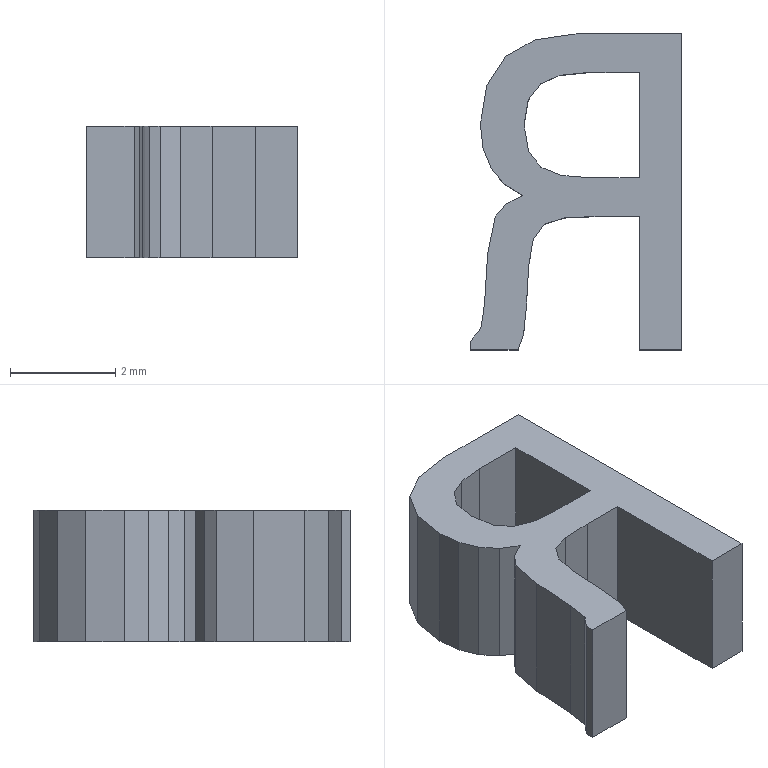Part | STEP file | lll_id1146_x_t | 1 solid | 41 faces | box 4.011 x 6 x 2.5 mm | volume 30.988 mm3 | plane 41
STEP:
#1=CARTESIAN_POINT('',(388.453,102.132,2.35));
#2=VERTEX_POINT('',#1);
#3=CARTESIAN_POINT('',(388.219,101.83,2.35));
#4=VERTEX_POINT('',#3);
#5=CARTESIAN_POINT('',(388.453,102.132,2.35));
#6=DIRECTION('',(-0.6108,-0.7918,0.));
#7=VECTOR('',#6,1.);
#8=LINE('',#5,#7);
#9=EDGE_CURVE('',#2,#4,#8,.T.);
#10=ORIENTED_EDGE('',*,*,#9,.T.);
#11=CARTESIAN_POINT('',(388.219,101.83,-0.15));
#12=VERTEX_POINT('',#11);
#13=CARTESIAN_POINT('',(388.219,101.83,-0.15));
#14=DIRECTION('',(0.,0.,1.));
#15=VECTOR('',#14,1.);
#16=LINE('',#13,#15);
#17=EDGE_CURVE('',#12,#4,#16,.T.);
#18=ORIENTED_EDGE('',*,*,#17,.F.);
#19=CARTESIAN_POINT('',(388.453,102.132,-0.15));
#20=VERTEX_POINT('',#19);
#21=CARTESIAN_POINT('',(388.453,102.132,-0.15));
#22=DIRECTION('',(-0.6108,-0.7918,0.));
#23=VECTOR('',#22,1.);
#24=LINE('',#21,#23);
#25=EDGE_CURVE('',#20,#12,#24,.T.);
#26=ORIENTED_EDGE('',*,*,#25,.F.);
#27=CARTESIAN_POINT('',(388.453,102.132,-0.15));
#28=DIRECTION('',(0.,0.,1.));
#29=VECTOR('',#28,1.);
#30=LINE('',#27,#29);
#31=EDGE_CURVE('',#20,#2,#30,.T.);
#32=ORIENTED_EDGE('',*,*,#31,.T.);
#33=EDGE_LOOP('',(#10,#18,#26,#32));
#34=FACE_OUTER_BOUND('',#33,.T.);
#35=CARTESIAN_POINT('',(388.453,102.132,-0.15));
#36=DIRECTION('',(-0.7918,0.6108,0.));
#37=DIRECTION('',(0.6108,0.7918,0.));
#38=AXIS2_PLACEMENT_3D('',#35,#36,#37);
#39=PLANE('',#38);
#40=ADVANCED_FACE('',(#34),#39,.F.);
#41=CARTESIAN_POINT('',(388.825,102.296,2.35));
#42=VERTEX_POINT('',#41);
#43=CARTESIAN_POINT('',(388.825,102.296,2.35));
#44=DIRECTION('',(-0.9147,-0.4042,0.));
#45=VECTOR('',#44,1.);
#46=LINE('',#43,#45);
#47=EDGE_CURVE('',#42,#2,#46,.T.);
#48=ORIENTED_EDGE('',*,*,#47,.T.);
#49=ORIENTED_EDGE('',*,*,#31,.F.);
#50=CARTESIAN_POINT('',(388.825,102.296,-0.15));
#51=VERTEX_POINT('',#50);
#52=CARTESIAN_POINT('',(388.825,102.296,-0.15));
#53=DIRECTION('',(-0.9147,-0.4042,0.));
#54=VECTOR('',#53,1.);
#55=LINE('',#52,#54);
#56=EDGE_CURVE('',#51,#20,#55,.T.);
#57=ORIENTED_EDGE('',*,*,#56,.F.);
#58=CARTESIAN_POINT('',(388.825,102.296,-0.15));
#59=DIRECTION('',(0.,0.,1.));
#60=VECTOR('',#59,1.);
#61=LINE('',#58,#60);
#62=EDGE_CURVE('',#51,#42,#61,.T.);
#63=ORIENTED_EDGE('',*,*,#62,.T.);
#64=EDGE_LOOP('',(#48,#49,#57,#63));
#65=FACE_OUTER_BOUND('',#64,.T.);
#66=CARTESIAN_POINT('',(388.825,102.296,-0.15));
#67=DIRECTION('',(-0.4042,0.9147,0.));
#68=DIRECTION('',(0.9147,0.4042,0.));
#69=AXIS2_PLACEMENT_3D('',#66,#67,#68);
#70=PLANE('',#69);
#71=ADVANCED_FACE('',(#65),#70,.F.);
#72=CARTESIAN_POINT('',(389.352,102.348,2.35));
#73=VERTEX_POINT('',#72);
#74=CARTESIAN_POINT('',(389.352,102.348,2.35));
#75=DIRECTION('',(-0.9952,-0.0979,0.));
#76=VECTOR('',#75,1.);
#77=LINE('',#74,#76);
#78=EDGE_CURVE('',#73,#42,#77,.T.);
#79=ORIENTED_EDGE('',*,*,#78,.T.);
#80=ORIENTED_EDGE('',*,*,#62,.F.);
#81=CARTESIAN_POINT('',(389.352,102.348,-0.15));
#82=VERTEX_POINT('',#81);
#83=CARTESIAN_POINT('',(389.352,102.348,-0.15));
#84=DIRECTION('',(-0.9952,-0.0979,0.));
#85=VECTOR('',#84,1.);
#86=LINE('',#83,#85);
#87=EDGE_CURVE('',#82,#51,#86,.T.);
#88=ORIENTED_EDGE('',*,*,#87,.F.);
#89=CARTESIAN_POINT('',(389.352,102.348,-0.15));
#90=DIRECTION('',(0.,0.,1.));
#91=VECTOR('',#90,1.);
#92=LINE('',#89,#91);
#93=EDGE_CURVE('',#82,#73,#92,.T.);
#94=ORIENTED_EDGE('',*,*,#93,.T.);
#95=EDGE_LOOP('',(#79,#80,#88,#94));
#96=FACE_OUTER_BOUND('',#95,.T.);
#97=CARTESIAN_POINT('',(389.352,102.348,-0.15));
#98=DIRECTION('',(-0.0979,0.9952,0.));
#99=DIRECTION('',(0.9952,0.0979,0.));
#100=AXIS2_PLACEMENT_3D('',#97,#98,#99);
#101=PLANE('',#100);
#102=ADVANCED_FACE('',(#96),#101,.F.);
#103=CARTESIAN_POINT('',(390.329,102.348,2.35));
#104=VERTEX_POINT('',#103);
#105=CARTESIAN_POINT('',(390.329,102.348,2.35));
#106=DIRECTION('',(-1.,0.,0.));
#107=VECTOR('',#106,1.);
#108=LINE('',#105,#107);
#109=EDGE_CURVE('',#104,#73,#108,.T.);
#110=ORIENTED_EDGE('',*,*,#109,.T.);
#111=ORIENTED_EDGE('',*,*,#93,.F.);
#112=CARTESIAN_POINT('',(390.329,102.348,-0.15));
#113=VERTEX_POINT('',#112);
#114=CARTESIAN_POINT('',(390.329,102.348,-0.15));
#115=DIRECTION('',(-1.,0.,0.));
#116=VECTOR('',#115,1.);
#117=LINE('',#114,#116);
#118=EDGE_CURVE('',#113,#82,#117,.T.);
#119=ORIENTED_EDGE('',*,*,#118,.F.);
#120=CARTESIAN_POINT('',(390.329,102.348,-0.15));
#121=DIRECTION('',(0.,0.,1.));
#122=VECTOR('',#121,1.);
#123=LINE('',#120,#122);
#124=EDGE_CURVE('',#113,#104,#123,.T.);
#125=ORIENTED_EDGE('',*,*,#124,.T.);
#126=EDGE_LOOP('',(#110,#111,#119,#125));
#127=FACE_OUTER_BOUND('',#126,.T.);
#128=CARTESIAN_POINT('',(390.329,102.348,-0.15));
#129=DIRECTION('',(0.,1.,0.));
#130=DIRECTION('',(0.,0.,1.));
#131=AXIS2_PLACEMENT_3D('',#128,#129,#130);
#132=PLANE('',#131);
#133=ADVANCED_FACE('',(#127),#132,.F.);
#134=CARTESIAN_POINT('',(390.329,100.351,2.35));
#135=VERTEX_POINT('',#134);
#136=CARTESIAN_POINT('',(390.329,100.351,2.35));
#137=DIRECTION('',(0.,1.,0.));
#138=VECTOR('',#137,1.);
#139=LINE('',#136,#138);
#140=EDGE_CURVE('',#135,#104,#139,.T.);
#141=ORIENTED_EDGE('',*,*,#140,.T.);
#142=ORIENTED_EDGE('',*,*,#124,.F.);
#143=CARTESIAN_POINT('',(390.329,100.351,-0.15));
#144=VERTEX_POINT('',#143);
#145=CARTESIAN_POINT('',(390.329,100.351,-0.15));
#146=DIRECTION('',(0.,1.,0.));
#147=VECTOR('',#146,1.);
#148=LINE('',#145,#147);
#149=EDGE_CURVE('',#144,#113,#148,.T.);
#150=ORIENTED_EDGE('',*,*,#149,.F.);
#151=CARTESIAN_POINT('',(390.329,100.351,-0.15));
#152=DIRECTION('',(0.,0.,1.));
#153=VECTOR('',#152,1.);
#154=LINE('',#151,#153);
#155=EDGE_CURVE('',#144,#135,#154,.T.);
#156=ORIENTED_EDGE('',*,*,#155,.T.);
#157=EDGE_LOOP('',(#141,#142,#150,#156));
#158=FACE_OUTER_BOUND('',#157,.T.);
#159=CARTESIAN_POINT('',(390.329,100.351,-0.15));
#160=DIRECTION('',(1.,0.,0.));
#161=DIRECTION('',(0.,0.,-1.));
#162=AXIS2_PLACEMENT_3D('',#159,#160,#161);
#163=PLANE('',#162);
#164=ADVANCED_FACE('',(#158),#163,.F.);
#165=CARTESIAN_POINT('',(389.404,100.351,2.35));
#166=VERTEX_POINT('',#165);
#167=CARTESIAN_POINT('',(389.404,100.351,2.35));
#168=DIRECTION('',(1.,0.,0.));
#169=VECTOR('',#168,1.);
#170=LINE('',#167,#169);
#171=EDGE_CURVE('',#166,#135,#170,.T.);
#172=ORIENTED_EDGE('',*,*,#171,.T.);
#173=ORIENTED_EDGE('',*,*,#155,.F.);
#174=CARTESIAN_POINT('',(389.404,100.351,-0.15));
#175=VERTEX_POINT('',#174);
#176=CARTESIAN_POINT('',(389.404,100.351,-0.15));
#177=DIRECTION('',(1.,0.,0.));
#178=VECTOR('',#177,1.);
#179=LINE('',#176,#178);
#180=EDGE_CURVE('',#175,#144,#179,.T.);
#181=ORIENTED_EDGE('',*,*,#180,.F.);
#182=CARTESIAN_POINT('',(389.404,100.351,-0.15));
#183=DIRECTION('',(0.,0.,1.));
#184=VECTOR('',#183,1.);
#185=LINE('',#182,#184);
#186=EDGE_CURVE('',#175,#166,#185,.T.);
#187=ORIENTED_EDGE('',*,*,#186,.T.);
#188=EDGE_LOOP('',(#172,#173,#181,#187));
#189=FACE_OUTER_BOUND('',#188,.T.);
#190=CARTESIAN_POINT('',(389.404,100.351,-0.15));
#191=DIRECTION('',(0.,-1.,0.));
#192=DIRECTION('',(0.,0.,-1.));
#193=AXIS2_PLACEMENT_3D('',#190,#191,#192);
#194=PLANE('',#193);
#195=ADVANCED_FACE('',(#189),#194,.F.);
#196=CARTESIAN_POINT('',(388.859,100.394,2.35));
#197=VERTEX_POINT('',#196);
#198=CARTESIAN_POINT('',(388.859,100.394,2.35));
#199=DIRECTION('',(0.9969,-0.07914,0.));
#200=VECTOR('',#199,1.);
#201=LINE('',#198,#200);
#202=EDGE_CURVE('',#197,#166,#201,.T.);
#203=ORIENTED_EDGE('',*,*,#202,.T.);
#204=ORIENTED_EDGE('',*,*,#186,.F.);
#205=CARTESIAN_POINT('',(388.859,100.394,-0.15));
#206=VERTEX_POINT('',#205);
#207=CARTESIAN_POINT('',(388.859,100.394,-0.15));
#208=DIRECTION('',(0.9969,-0.07914,0.));
#209=VECTOR('',#208,1.);
#210=LINE('',#207,#209);
#211=EDGE_CURVE('',#206,#175,#210,.T.);
#212=ORIENTED_EDGE('',*,*,#211,.F.);
#213=CARTESIAN_POINT('',(388.859,100.394,-0.15));
#214=DIRECTION('',(0.,0.,1.));
#215=VECTOR('',#214,1.);
#216=LINE('',#213,#215);
#217=EDGE_CURVE('',#206,#197,#216,.T.);
#218=ORIENTED_EDGE('',*,*,#217,.T.);
#219=EDGE_LOOP('',(#203,#204,#212,#218));
#220=FACE_OUTER_BOUND('',#219,.T.);
#221=CARTESIAN_POINT('',(388.859,100.394,-0.15));
#222=DIRECTION('',(-0.07914,-0.9969,0.));
#223=DIRECTION('',(-0.9969,0.07914,0.));
#224=AXIS2_PLACEMENT_3D('',#221,#222,#223);
#225=PLANE('',#224);
#226=ADVANCED_FACE('',(#220),#225,.F.);
#227=CARTESIAN_POINT('',(388.461,100.55,2.35));
#228=VERTEX_POINT('',#227);
#229=CARTESIAN_POINT('',(388.461,100.55,2.35));
#230=DIRECTION('',(0.9313,-0.3644,0.));
#231=VECTOR('',#230,1.);
#232=LINE('',#229,#231);
#233=EDGE_CURVE('',#228,#197,#232,.T.);
#234=ORIENTED_EDGE('',*,*,#233,.T.);
#235=ORIENTED_EDGE('',*,*,#217,.F.);
#236=CARTESIAN_POINT('',(388.461,100.55,-0.15));
#237=VERTEX_POINT('',#236);
#238=CARTESIAN_POINT('',(388.461,100.55,-0.15));
#239=DIRECTION('',(0.9313,-0.3644,0.));
#240=VECTOR('',#239,1.);
#241=LINE('',#238,#240);
#242=EDGE_CURVE('',#237,#206,#241,.T.);
#243=ORIENTED_EDGE('',*,*,#242,.F.);
#244=CARTESIAN_POINT('',(388.461,100.55,-0.15));
#245=DIRECTION('',(0.,0.,1.));
#246=VECTOR('',#245,1.);
#247=LINE('',#244,#246);
#248=EDGE_CURVE('',#237,#228,#247,.T.);
#249=ORIENTED_EDGE('',*,*,#248,.T.);
#250=EDGE_LOOP('',(#234,#235,#243,#249));
#251=FACE_OUTER_BOUND('',#250,.T.);
#252=CARTESIAN_POINT('',(388.461,100.55,-0.15));
#253=DIRECTION('',(-0.3644,-0.9313,0.));
#254=DIRECTION('',(-0.9313,0.3644,0.));
#255=AXIS2_PLACEMENT_3D('',#252,#253,#254);
#256=PLANE('',#255);
#257=ADVANCED_FACE('',(#251),#256,.F.);
#258=CARTESIAN_POINT('',(388.228,100.853,2.35));
#259=VERTEX_POINT('',#258);
#260=CARTESIAN_POINT('',(388.228,100.853,2.35));
#261=DIRECTION('',(0.6108,-0.7918,0.));
#262=VECTOR('',#261,1.);
#263=LINE('',#260,#262);
#264=EDGE_CURVE('',#259,#228,#263,.T.);
#265=ORIENTED_EDGE('',*,*,#264,.T.);
#266=ORIENTED_EDGE('',*,*,#248,.F.);
#267=CARTESIAN_POINT('',(388.228,100.853,-0.15));
#268=VERTEX_POINT('',#267);
#269=CARTESIAN_POINT('',(388.228,100.853,-0.15));
#270=DIRECTION('',(0.6108,-0.7918,0.));
#271=VECTOR('',#270,1.);
#272=LINE('',#269,#271);
#273=EDGE_CURVE('',#268,#237,#272,.T.);
#274=ORIENTED_EDGE('',*,*,#273,.F.);
#275=CARTESIAN_POINT('',(388.228,100.853,-0.15));
#276=DIRECTION('',(0.,0.,1.));
#277=VECTOR('',#276,1.);
#278=LINE('',#275,#277);
#279=EDGE_CURVE('',#268,#259,#278,.T.);
#280=ORIENTED_EDGE('',*,*,#279,.T.);
#281=EDGE_LOOP('',(#265,#266,#274,#280));
#282=FACE_OUTER_BOUND('',#281,.T.);
#283=CARTESIAN_POINT('',(388.228,100.853,-0.15));
#284=DIRECTION('',(-0.7918,-0.6108,0.));
#285=DIRECTION('',(-0.6108,0.7918,0.));
#286=AXIS2_PLACEMENT_3D('',#283,#284,#285);
#287=PLANE('',#286);
#288=ADVANCED_FACE('',(#282),#287,.F.);
#289=CARTESIAN_POINT('',(388.142,101.354,2.35));
#290=VERTEX_POINT('',#289);
#291=CARTESIAN_POINT('',(388.142,101.354,2.35));
#292=DIRECTION('',(0.17,-0.9855,0.));
#293=VECTOR('',#292,1.);
#294=LINE('',#291,#293);
#295=EDGE_CURVE('',#290,#259,#294,.T.);
#296=ORIENTED_EDGE('',*,*,#295,.T.);
#297=ORIENTED_EDGE('',*,*,#279,.F.);
#298=CARTESIAN_POINT('',(388.142,101.354,-0.15));
#299=VERTEX_POINT('',#298);
#300=CARTESIAN_POINT('',(388.142,101.354,-0.15));
#301=DIRECTION('',(0.17,-0.9855,0.));
#302=VECTOR('',#301,1.);
#303=LINE('',#300,#302);
#304=EDGE_CURVE('',#299,#268,#303,.T.);
#305=ORIENTED_EDGE('',*,*,#304,.F.);
#306=CARTESIAN_POINT('',(388.142,101.354,-0.15));
#307=DIRECTION('',(0.,0.,1.));
#308=VECTOR('',#307,1.);
#309=LINE('',#306,#308);
#310=EDGE_CURVE('',#299,#290,#309,.T.);
#311=ORIENTED_EDGE('',*,*,#310,.T.);
#312=EDGE_LOOP('',(#296,#297,#305,#311));
#313=FACE_OUTER_BOUND('',#312,.T.);
#314=CARTESIAN_POINT('',(388.142,101.354,-0.15));
#315=DIRECTION('',(-0.9855,-0.17,0.));
#316=DIRECTION('',(-0.17,0.9855,0.));
#317=AXIS2_PLACEMENT_3D('',#314,#315,#316);
#318=PLANE('',#317);
#319=ADVANCED_FACE('',(#313),#318,.F.);
#320=CARTESIAN_POINT('',(387.121,97.247,2.35));
#321=VERTEX_POINT('',#320);
#322=CARTESIAN_POINT('',(387.121,97.083,2.35));
#323=VERTEX_POINT('',#322);
#324=CARTESIAN_POINT('',(387.121,97.247,2.35));
#325=DIRECTION('',(0.,-1.,0.));
#326=VECTOR('',#325,1.);
#327=LINE('',#324,#326);
#328=EDGE_CURVE('',#321,#323,#327,.T.);
#329=ORIENTED_EDGE('',*,*,#328,.F.);
#330=CARTESIAN_POINT('',(387.121,97.247,-0.15));
#331=VERTEX_POINT('',#330);
#332=CARTESIAN_POINT('',(387.121,97.247,-0.15));
#333=DIRECTION('',(0.,0.,1.));
#334=VECTOR('',#333,1.);
#335=LINE('',#332,#334);
#336=EDGE_CURVE('',#331,#321,#335,.T.);
#337=ORIENTED_EDGE('',*,*,#336,.F.);
#338=CARTESIAN_POINT('',(387.121,97.083,-0.15));
#339=VERTEX_POINT('',#338);
#340=CARTESIAN_POINT('',(387.121,97.247,-0.15));
#341=DIRECTION('',(0.,-1.,0.));
#342=VECTOR('',#341,1.);
#343=LINE('',#340,#342);
#344=EDGE_CURVE('',#331,#339,#343,.T.);
#345=ORIENTED_EDGE('',*,*,#344,.T.);
#346=CARTESIAN_POINT('',(387.121,97.083,-0.15));
#347=DIRECTION('',(0.,0.,1.));
#348=VECTOR('',#347,1.);
#349=LINE('',#346,#348);
#350=EDGE_CURVE('',#339,#323,#349,.T.);
#351=ORIENTED_EDGE('',*,*,#350,.T.);
#352=EDGE_LOOP('',(#329,#337,#345,#351));
#353=FACE_OUTER_BOUND('',#352,.T.);
#354=CARTESIAN_POINT('',(387.121,97.247,-0.15));
#355=DIRECTION('',(-1.,0.,0.));
#356=DIRECTION('',(0.,0.,1.));
#357=AXIS2_PLACEMENT_3D('',#354,#355,#356);
#358=PLANE('',#357);
#359=ADVANCED_FACE('',(#353),#358,.T.);
#360=CARTESIAN_POINT('',(388.029,97.083,2.35));
#361=VERTEX_POINT('',#360);
#362=CARTESIAN_POINT('',(387.121,97.083,2.35));
#363=DIRECTION('',(1.,0.,0.));
#364=VECTOR('',#363,1.);
#365=LINE('',#362,#364);
#366=EDGE_CURVE('',#323,#361,#365,.T.);
#367=ORIENTED_EDGE('',*,*,#366,.F.);
#368=ORIENTED_EDGE('',*,*,#350,.F.);
#369=CARTESIAN_POINT('',(388.029,97.083,-0.15));
#370=VERTEX_POINT('',#369);
#371=CARTESIAN_POINT('',(387.121,97.083,-0.15));
#372=DIRECTION('',(1.,0.,0.));
#373=VECTOR('',#372,1.);
#374=LINE('',#371,#373);
#375=EDGE_CURVE('',#339,#370,#374,.T.);
#376=ORIENTED_EDGE('',*,*,#375,.T.);
#377=CARTESIAN_POINT('',(388.029,97.083,-0.15));
#378=DIRECTION('',(0.,0.,1.));
#379=VECTOR('',#378,1.);
#380=LINE('',#377,#379);
#381=EDGE_CURVE('',#370,#361,#380,.T.);
#382=ORIENTED_EDGE('',*,*,#381,.T.);
#383=EDGE_LOOP('',(#367,#368,#376,#382));
#384=FACE_OUTER_BOUND('',#383,.T.);
#385=CARTESIAN_POINT('',(387.121,97.083,-0.15));
#386=DIRECTION('',(0.,-1.,0.));
#387=DIRECTION('',(0.,0.,-1.));
#388=AXIS2_PLACEMENT_3D('',#385,#386,#387);
#389=PLANE('',#388);
#390=ADVANCED_FACE('',(#384),#389,.T.);
#391=CARTESIAN_POINT('',(388.133,97.386,2.35));
#392=VERTEX_POINT('',#391);
#393=CARTESIAN_POINT('',(388.029,97.083,2.35));
#394=DIRECTION('',(0.3242,0.946,0.));
#395=VECTOR('',#394,1.);
#396=LINE('',#393,#395);
#397=EDGE_CURVE('',#361,#392,#396,.T.);
#398=ORIENTED_EDGE('',*,*,#397,.F.);
#399=ORIENTED_EDGE('',*,*,#381,.F.);
#400=CARTESIAN_POINT('',(388.133,97.386,-0.15));
#401=VERTEX_POINT('',#400);
#402=CARTESIAN_POINT('',(388.029,97.083,-0.15));
#403=DIRECTION('',(0.3242,0.946,0.));
#404=VECTOR('',#403,1.);
#405=LINE('',#402,#404);
#406=EDGE_CURVE('',#370,#401,#405,.T.);
#407=ORIENTED_EDGE('',*,*,#406,.T.);
#408=CARTESIAN_POINT('',(388.133,97.386,-0.15));
#409=DIRECTION('',(0.,0.,1.));
#410=VECTOR('',#409,1.);
#411=LINE('',#408,#410);
#412=EDGE_CURVE('',#401,#392,#411,.T.);
#413=ORIENTED_EDGE('',*,*,#412,.T.);
#414=EDGE_LOOP('',(#398,#399,#407,#413));
#415=FACE_OUTER_BOUND('',#414,.T.);
#416=CARTESIAN_POINT('',(388.029,97.083,-0.15));
#417=DIRECTION('',(0.946,-0.3242,0.));
#418=DIRECTION('',(-0.3242,-0.946,0.));
#419=AXIS2_PLACEMENT_3D('',#416,#417,#418);
#420=PLANE('',#419);
#421=ADVANCED_FACE('',(#415),#420,.T.);
#422=CARTESIAN_POINT('',(388.185,97.896,2.35));
#423=VERTEX_POINT('',#422);
#424=CARTESIAN_POINT('',(388.133,97.386,2.35));
#425=DIRECTION('',(0.1012,0.9949,0.));
#426=VECTOR('',#425,1.);
#427=LINE('',#424,#426);
#428=EDGE_CURVE('',#392,#423,#427,.T.);
#429=ORIENTED_EDGE('',*,*,#428,.F.);
#430=ORIENTED_EDGE('',*,*,#412,.F.);
#431=CARTESIAN_POINT('',(388.185,97.896,-0.15));
#432=VERTEX_POINT('',#431);
#433=CARTESIAN_POINT('',(388.133,97.386,-0.15));
#434=DIRECTION('',(0.1012,0.9949,0.));
#435=VECTOR('',#434,1.);
#436=LINE('',#433,#435);
#437=EDGE_CURVE('',#401,#432,#436,.T.);
#438=ORIENTED_EDGE('',*,*,#437,.T.);
#439=CARTESIAN_POINT('',(388.185,97.896,-0.15));
#440=DIRECTION('',(0.,0.,1.));
#441=VECTOR('',#440,1.);
#442=LINE('',#439,#441);
#443=EDGE_CURVE('',#432,#423,#442,.T.);
#444=ORIENTED_EDGE('',*,*,#443,.T.);
#445=EDGE_LOOP('',(#429,#430,#438,#444));
#446=FACE_OUTER_BOUND('',#445,.T.);
#447=CARTESIAN_POINT('',(388.133,97.386,-0.15));
#448=DIRECTION('',(0.9949,-0.1012,0.));
#449=DIRECTION('',(-0.1012,-0.9949,0.));
#450=AXIS2_PLACEMENT_3D('',#447,#448,#449);
#451=PLANE('',#450);
#452=ADVANCED_FACE('',(#446),#451,.T.);
#453=CARTESIAN_POINT('',(388.228,98.674,2.35));
#454=VERTEX_POINT('',#453);
#455=CARTESIAN_POINT('',(388.185,97.896,2.35));
#456=DIRECTION('',(0.05553,0.9985,0.));
#457=VECTOR('',#456,1.);
#458=LINE('',#455,#457);
#459=EDGE_CURVE('',#423,#454,#458,.T.);
#460=ORIENTED_EDGE('',*,*,#459,.F.);
#461=ORIENTED_EDGE('',*,*,#443,.F.);
#462=CARTESIAN_POINT('',(388.228,98.674,-0.15));
#463=VERTEX_POINT('',#462);
#464=CARTESIAN_POINT('',(388.185,97.896,-0.15));
#465=DIRECTION('',(0.05553,0.9985,0.));
#466=VECTOR('',#465,1.);
#467=LINE('',#464,#466);
#468=EDGE_CURVE('',#432,#463,#467,.T.);
#469=ORIENTED_EDGE('',*,*,#468,.T.);
#470=CARTESIAN_POINT('',(388.228,98.674,-0.15));
#471=DIRECTION('',(0.,0.,1.));
#472=VECTOR('',#471,1.);
#473=LINE('',#470,#472);
#474=EDGE_CURVE('',#463,#454,#473,.T.);
#475=ORIENTED_EDGE('',*,*,#474,.T.);
#476=EDGE_LOOP('',(#460,#461,#469,#475));
#477=FACE_OUTER_BOUND('',#476,.T.);
#478=CARTESIAN_POINT('',(388.185,97.896,-0.15));
#479=DIRECTION('',(0.9985,-0.05553,0.));
#480=DIRECTION('',(-0.05553,-0.9985,0.));
#481=AXIS2_PLACEMENT_3D('',#478,#479,#480);
#482=PLANE('',#481);
#483=ADVANCED_FACE('',(#477),#482,.T.);
#484=CARTESIAN_POINT('',(388.314,99.184,2.35));
#485=VERTEX_POINT('',#484);
#486=CARTESIAN_POINT('',(388.228,98.674,2.35));
#487=DIRECTION('',(0.1671,0.9859,0.));
#488=VECTOR('',#487,1.);
#489=LINE('',#486,#488);
#490=EDGE_CURVE('',#454,#485,#489,.T.);
#491=ORIENTED_EDGE('',*,*,#490,.F.);
#492=ORIENTED_EDGE('',*,*,#474,.F.);
#493=CARTESIAN_POINT('',(388.314,99.184,-0.15));
#494=VERTEX_POINT('',#493);
#495=CARTESIAN_POINT('',(388.228,98.674,-0.15));
#496=DIRECTION('',(0.1671,0.9859,0.));
#497=VECTOR('',#496,1.);
#498=LINE('',#495,#497);
#499=EDGE_CURVE('',#463,#494,#498,.T.);
#500=ORIENTED_EDGE('',*,*,#499,.T.);
#501=CARTESIAN_POINT('',(388.314,99.184,-0.15));
#502=DIRECTION('',(0.,0.,1.));
#503=VECTOR('',#502,1.);
#504=LINE('',#501,#503);
#505=EDGE_CURVE('',#494,#485,#504,.T.);
#506=ORIENTED_EDGE('',*,*,#505,.T.);
#507=EDGE_LOOP('',(#491,#492,#500,#506));
#508=FACE_OUTER_BOUND('',#507,.T.);
#509=CARTESIAN_POINT('',(388.228,98.674,-0.15));
#510=DIRECTION('',(0.9859,-0.1671,0.));
#511=DIRECTION('',(-0.1671,-0.9859,0.));
#512=AXIS2_PLACEMENT_3D('',#509,#510,#511);
#513=PLANE('',#512);
#514=ADVANCED_FACE('',(#508),#513,.T.);
#515=CARTESIAN_POINT('',(388.522,99.469,2.35));
#516=VERTEX_POINT('',#515);
#517=CARTESIAN_POINT('',(388.314,99.184,2.35));
#518=DIRECTION('',(0.5882,0.8087,0.));
#519=VECTOR('',#518,1.);
#520=LINE('',#517,#519);
#521=EDGE_CURVE('',#485,#516,#520,.T.);
#522=ORIENTED_EDGE('',*,*,#521,.F.);
#523=ORIENTED_EDGE('',*,*,#505,.F.);
#524=CARTESIAN_POINT('',(388.522,99.469,-0.15));
#525=VERTEX_POINT('',#524);
#526=CARTESIAN_POINT('',(388.314,99.184,-0.15));
#527=DIRECTION('',(0.5882,0.8087,0.));
#528=VECTOR('',#527,1.);
#529=LINE('',#526,#528);
#530=EDGE_CURVE('',#494,#525,#529,.T.);
#531=ORIENTED_EDGE('',*,*,#530,.T.);
#532=CARTESIAN_POINT('',(388.522,99.469,-0.15));
#533=DIRECTION('',(0.,0.,1.));
#534=VECTOR('',#533,1.);
#535=LINE('',#532,#534);
#536=EDGE_CURVE('',#525,#516,#535,.T.);
#537=ORIENTED_EDGE('',*,*,#536,.T.);
#538=EDGE_LOOP('',(#522,#523,#531,#537));
#539=FACE_OUTER_BOUND('',#538,.T.);
#540=CARTESIAN_POINT('',(388.314,99.184,-0.15));
#541=DIRECTION('',(0.8087,-0.5882,0.));
#542=DIRECTION('',(-0.5882,-0.8087,0.));
#543=AXIS2_PLACEMENT_3D('',#540,#541,#542);
#544=PLANE('',#543);
#545=ADVANCED_FACE('',(#539),#544,.T.);
#546=CARTESIAN_POINT('',(388.902,99.59,2.35));
#547=VERTEX_POINT('',#546);
#548=CARTESIAN_POINT('',(388.522,99.469,2.35));
#549=DIRECTION('',(0.9529,0.3032,0.));
#550=VECTOR('',#549,1.);
#551=LINE('',#548,#550);
#552=EDGE_CURVE('',#516,#547,#551,.T.);
#553=ORIENTED_EDGE('',*,*,#552,.F.);
#554=ORIENTED_EDGE('',*,*,#536,.F.);
#555=CARTESIAN_POINT('',(388.902,99.59,-0.15));
#556=VERTEX_POINT('',#555);
#557=CARTESIAN_POINT('',(388.522,99.469,-0.15));
#558=DIRECTION('',(0.9529,0.3032,0.));
#559=VECTOR('',#558,1.);
#560=LINE('',#557,#559);
#561=EDGE_CURVE('',#525,#556,#560,.T.);
#562=ORIENTED_EDGE('',*,*,#561,.T.);
#563=CARTESIAN_POINT('',(388.902,99.59,-0.15));
#564=DIRECTION('',(0.,0.,1.));
#565=VECTOR('',#564,1.);
#566=LINE('',#563,#565);
#567=EDGE_CURVE('',#556,#547,#566,.T.);
#568=ORIENTED_EDGE('',*,*,#567,.T.);
#569=EDGE_LOOP('',(#553,#554,#562,#568));
#570=FACE_OUTER_BOUND('',#569,.T.);
#571=CARTESIAN_POINT('',(388.522,99.469,-0.15));
#572=DIRECTION('',(0.3032,-0.9529,0.));
#573=DIRECTION('',(-0.9529,-0.3032,0.));
#574=AXIS2_PLACEMENT_3D('',#571,#572,#573);
#575=PLANE('',#574);
#576=ADVANCED_FACE('',(#570),#575,.T.);
#577=CARTESIAN_POINT('',(389.508,99.616,2.35));
#578=VERTEX_POINT('',#577);
#579=CARTESIAN_POINT('',(388.902,99.59,2.35));
#580=DIRECTION('',(0.9991,0.04282,0.));
#581=VECTOR('',#580,1.);
#582=LINE('',#579,#581);
#583=EDGE_CURVE('',#547,#578,#582,.T.);
#584=ORIENTED_EDGE('',*,*,#583,.F.);
#585=ORIENTED_EDGE('',*,*,#567,.F.);
#586=CARTESIAN_POINT('',(389.508,99.616,-0.15));
#587=VERTEX_POINT('',#586);
#588=CARTESIAN_POINT('',(388.902,99.59,-0.15));
#589=DIRECTION('',(0.9991,0.04282,0.));
#590=VECTOR('',#589,1.);
#591=LINE('',#588,#590);
#592=EDGE_CURVE('',#556,#587,#591,.T.);
#593=ORIENTED_EDGE('',*,*,#592,.T.);
#594=CARTESIAN_POINT('',(389.508,99.616,-0.15));
#595=DIRECTION('',(0.,0.,1.));
#596=VECTOR('',#595,1.);
#597=LINE('',#594,#596);
#598=EDGE_CURVE('',#587,#578,#597,.T.);
#599=ORIENTED_EDGE('',*,*,#598,.T.);
#600=EDGE_LOOP('',(#584,#585,#593,#599));
#601=FACE_OUTER_BOUND('',#600,.T.);
#602=CARTESIAN_POINT('',(388.902,99.59,-0.15));
#603=DIRECTION('',(0.04282,-0.9991,0.));
#604=DIRECTION('',(-0.9991,-0.04282,0.));
#605=AXIS2_PLACEMENT_3D('',#602,#603,#604);
#606=PLANE('',#605);
#607=ADVANCED_FACE('',(#601),#606,.T.);
#608=CARTESIAN_POINT('',(390.329,99.616,2.35));
#609=VERTEX_POINT('',#608);
#610=CARTESIAN_POINT('',(389.508,99.616,2.35));
#611=DIRECTION('',(1.,0.,0.));
#612=VECTOR('',#611,1.);
#613=LINE('',#610,#612);
#614=EDGE_CURVE('',#578,#609,#613,.T.);
#615=ORIENTED_EDGE('',*,*,#614,.F.);
#616=ORIENTED_EDGE('',*,*,#598,.F.);
#617=CARTESIAN_POINT('',(390.329,99.616,-0.15));
#618=VERTEX_POINT('',#617);
#619=CARTESIAN_POINT('',(389.508,99.616,-0.15));
#620=DIRECTION('',(1.,0.,0.));
#621=VECTOR('',#620,1.);
#622=LINE('',#619,#621);
#623=EDGE_CURVE('',#587,#618,#622,.T.);
#624=ORIENTED_EDGE('',*,*,#623,.T.);
#625=CARTESIAN_POINT('',(390.329,99.616,-0.15));
#626=DIRECTION('',(0.,0.,1.));
#627=VECTOR('',#626,1.);
#628=LINE('',#625,#627);
#629=EDGE_CURVE('',#618,#609,#628,.T.);
#630=ORIENTED_EDGE('',*,*,#629,.T.);
#631=EDGE_LOOP('',(#615,#616,#624,#630));
#632=FACE_OUTER_BOUND('',#631,.T.);
#633=CARTESIAN_POINT('',(389.508,99.616,-0.15));
#634=DIRECTION('',(0.,-1.,0.));
#635=DIRECTION('',(0.,0.,-1.));
#636=AXIS2_PLACEMENT_3D('',#633,#634,#635);
#637=PLANE('',#636);
#638=ADVANCED_FACE('',(#632),#637,.T.);
#639=CARTESIAN_POINT('',(390.329,97.083,2.35));
#640=VERTEX_POINT('',#639);
#641=CARTESIAN_POINT('',(390.329,99.616,2.35));
#642=DIRECTION('',(0.,-1.,0.));
#643=VECTOR('',#642,1.);
#644=LINE('',#641,#643);
#645=EDGE_CURVE('',#609,#640,#644,.T.);
#646=ORIENTED_EDGE('',*,*,#645,.F.);
#647=ORIENTED_EDGE('',*,*,#629,.F.);
#648=CARTESIAN_POINT('',(390.329,97.083,-0.15));
#649=VERTEX_POINT('',#648);
#650=CARTESIAN_POINT('',(390.329,99.616,-0.15));
#651=DIRECTION('',(0.,-1.,0.));
#652=VECTOR('',#651,1.);
#653=LINE('',#650,#652);
#654=EDGE_CURVE('',#618,#649,#653,.T.);
#655=ORIENTED_EDGE('',*,*,#654,.T.);
#656=CARTESIAN_POINT('',(390.329,97.083,-0.15));
#657=DIRECTION('',(0.,0.,1.));
#658=VECTOR('',#657,1.);
#659=LINE('',#656,#658);
#660=EDGE_CURVE('',#649,#640,#659,.T.);
#661=ORIENTED_EDGE('',*,*,#660,.T.);
#662=EDGE_LOOP('',(#646,#647,#655,#661));
#663=FACE_OUTER_BOUND('',#662,.T.);
#664=CARTESIAN_POINT('',(390.329,99.616,-0.15));
#665=DIRECTION('',(-1.,0.,0.));
#666=DIRECTION('',(0.,0.,1.));
#667=AXIS2_PLACEMENT_3D('',#664,#665,#666);
#668=PLANE('',#667);
#669=ADVANCED_FACE('',(#663),#668,.T.);
#670=CARTESIAN_POINT('',(391.133,97.083,2.35));
#671=VERTEX_POINT('',#670);
#672=CARTESIAN_POINT('',(390.329,97.083,2.35));
#673=DIRECTION('',(1.,0.,0.));
#674=VECTOR('',#673,1.);
#675=LINE('',#672,#674);
#676=EDGE_CURVE('',#640,#671,#675,.T.);
#677=ORIENTED_EDGE('',*,*,#676,.F.);
#678=ORIENTED_EDGE('',*,*,#660,.F.);
#679=CARTESIAN_POINT('',(391.133,97.083,-0.15));
#680=VERTEX_POINT('',#679);
#681=CARTESIAN_POINT('',(390.329,97.083,-0.15));
#682=DIRECTION('',(1.,0.,0.));
#683=VECTOR('',#682,1.);
#684=LINE('',#681,#683);
#685=EDGE_CURVE('',#649,#680,#684,.T.);
#686=ORIENTED_EDGE('',*,*,#685,.T.);
#687=CARTESIAN_POINT('',(391.133,97.083,-0.15));
#688=DIRECTION('',(0.,0.,1.));
#689=VECTOR('',#688,1.);
#690=LINE('',#687,#689);
#691=EDGE_CURVE('',#680,#671,#690,.T.);
#692=ORIENTED_EDGE('',*,*,#691,.T.);
#693=EDGE_LOOP('',(#677,#678,#686,#692));
#694=FACE_OUTER_BOUND('',#693,.T.);
#695=CARTESIAN_POINT('',(390.329,97.083,-0.15));
#696=DIRECTION('',(0.,-1.,0.));
#697=DIRECTION('',(0.,0.,-1.));
#698=AXIS2_PLACEMENT_3D('',#695,#696,#697);
#699=PLANE('',#698);
#700=ADVANCED_FACE('',(#694),#699,.T.);
#701=CARTESIAN_POINT('',(391.133,103.083,2.35));
#702=VERTEX_POINT('',#701);
#703=CARTESIAN_POINT('',(391.133,97.083,2.35));
#704=DIRECTION('',(0.,1.,0.));
#705=VECTOR('',#704,1.);
#706=LINE('',#703,#705);
#707=EDGE_CURVE('',#671,#702,#706,.T.);
#708=ORIENTED_EDGE('',*,*,#707,.F.);
#709=ORIENTED_EDGE('',*,*,#691,.F.);
#710=CARTESIAN_POINT('',(391.133,103.083,-0.15));
#711=VERTEX_POINT('',#710);
#712=CARTESIAN_POINT('',(391.133,97.083,-0.15));
#713=DIRECTION('',(0.,1.,0.));
#714=VECTOR('',#713,1.);
#715=LINE('',#712,#714);
#716=EDGE_CURVE('',#680,#711,#715,.T.);
#717=ORIENTED_EDGE('',*,*,#716,.T.);
#718=CARTESIAN_POINT('',(391.133,103.083,-0.15));
#719=DIRECTION('',(0.,0.,1.));
#720=VECTOR('',#719,1.);
#721=LINE('',#718,#720);
#722=EDGE_CURVE('',#711,#702,#721,.T.);
#723=ORIENTED_EDGE('',*,*,#722,.T.);
#724=EDGE_LOOP('',(#708,#709,#717,#723));
#725=FACE_OUTER_BOUND('',#724,.T.);
#726=CARTESIAN_POINT('',(391.133,97.083,-0.15));
#727=DIRECTION('',(1.,0.,0.));
#728=DIRECTION('',(0.,0.,-1.));
#729=AXIS2_PLACEMENT_3D('',#726,#727,#728);
#730=PLANE('',#729);
#731=ADVANCED_FACE('',(#725),#730,.T.);
#732=CARTESIAN_POINT('',(389.127,103.083,2.35));
#733=VERTEX_POINT('',#732);
#734=CARTESIAN_POINT('',(391.133,103.083,2.35));
#735=DIRECTION('',(-1.,0.,0.));
#736=VECTOR('',#735,1.);
#737=LINE('',#734,#736);
#738=EDGE_CURVE('',#702,#733,#737,.T.);
#739=ORIENTED_EDGE('',*,*,#738,.F.);
#740=ORIENTED_EDGE('',*,*,#722,.F.);
#741=CARTESIAN_POINT('',(389.127,103.083,-0.15));
#742=VERTEX_POINT('',#741);
#743=CARTESIAN_POINT('',(391.133,103.083,-0.15));
#744=DIRECTION('',(-1.,0.,0.));
#745=VECTOR('',#744,1.);
#746=LINE('',#743,#745);
#747=EDGE_CURVE('',#711,#742,#746,.T.);
#748=ORIENTED_EDGE('',*,*,#747,.T.);
#749=CARTESIAN_POINT('',(389.127,103.083,-0.15));
#750=DIRECTION('',(0.,0.,1.));
#751=VECTOR('',#750,1.);
#752=LINE('',#749,#751);
#753=EDGE_CURVE('',#742,#733,#752,.T.);
#754=ORIENTED_EDGE('',*,*,#753,.T.);
#755=EDGE_LOOP('',(#739,#740,#748,#754));
#756=FACE_OUTER_BOUND('',#755,.T.);
#757=CARTESIAN_POINT('',(391.133,103.083,-0.15));
#758=DIRECTION('',(0.,1.,0.));
#759=DIRECTION('',(0.,0.,1.));
#760=AXIS2_PLACEMENT_3D('',#757,#758,#759);
#761=PLANE('',#760);
#762=ADVANCED_FACE('',(#756),#761,.T.);
#763=CARTESIAN_POINT('',(388.349,102.971,2.35));
#764=VERTEX_POINT('',#763);
#765=CARTESIAN_POINT('',(389.127,103.083,2.35));
#766=DIRECTION('',(-0.9897,-0.143,0.));
#767=VECTOR('',#766,1.);
#768=LINE('',#765,#767);
#769=EDGE_CURVE('',#733,#764,#768,.T.);
#770=ORIENTED_EDGE('',*,*,#769,.F.);
#771=ORIENTED_EDGE('',*,*,#753,.F.);
#772=CARTESIAN_POINT('',(388.349,102.971,-0.15));
#773=VERTEX_POINT('',#772);
#774=CARTESIAN_POINT('',(389.127,103.083,-0.15));
#775=DIRECTION('',(-0.9897,-0.143,0.));
#776=VECTOR('',#775,1.);
#777=LINE('',#774,#776);
#778=EDGE_CURVE('',#742,#773,#777,.T.);
#779=ORIENTED_EDGE('',*,*,#778,.T.);
#780=CARTESIAN_POINT('',(388.349,102.971,-0.15));
#781=DIRECTION('',(0.,0.,1.));
#782=VECTOR('',#781,1.);
#783=LINE('',#780,#782);
#784=EDGE_CURVE('',#773,#764,#783,.T.);
#785=ORIENTED_EDGE('',*,*,#784,.T.);
#786=EDGE_LOOP('',(#770,#771,#779,#785));
#787=FACE_OUTER_BOUND('',#786,.T.);
#788=CARTESIAN_POINT('',(389.127,103.083,-0.15));
#789=DIRECTION('',(-0.143,0.9897,0.));
#790=DIRECTION('',(0.9897,0.143,0.));
#791=AXIS2_PLACEMENT_3D('',#788,#789,#790);
#792=PLANE('',#791);
#793=ADVANCED_FACE('',(#787),#792,.T.);
#794=CARTESIAN_POINT('',(387.778,102.642,2.35));
#795=VERTEX_POINT('',#794);
#796=CARTESIAN_POINT('',(388.349,102.971,2.35));
#797=DIRECTION('',(-0.8666,-0.4989,0.));
#798=VECTOR('',#797,1.);
#799=LINE('',#796,#798);
#800=EDGE_CURVE('',#764,#795,#799,.T.);
#801=ORIENTED_EDGE('',*,*,#800,.F.);
#802=ORIENTED_EDGE('',*,*,#784,.F.);
#803=CARTESIAN_POINT('',(387.778,102.642,-0.15));
#804=VERTEX_POINT('',#803);
#805=CARTESIAN_POINT('',(388.349,102.971,-0.15));
#806=DIRECTION('',(-0.8666,-0.4989,0.));
#807=VECTOR('',#806,1.);
#808=LINE('',#805,#807);
#809=EDGE_CURVE('',#773,#804,#808,.T.);
#810=ORIENTED_EDGE('',*,*,#809,.T.);
#811=CARTESIAN_POINT('',(387.778,102.642,-0.15));
#812=DIRECTION('',(0.,0.,1.));
#813=VECTOR('',#812,1.);
#814=LINE('',#811,#813);
#815=EDGE_CURVE('',#804,#795,#814,.T.);
#816=ORIENTED_EDGE('',*,*,#815,.T.);
#817=EDGE_LOOP('',(#801,#802,#810,#816));
#818=FACE_OUTER_BOUND('',#817,.T.);
#819=CARTESIAN_POINT('',(388.349,102.971,-0.15));
#820=DIRECTION('',(-0.4989,0.8666,0.));
#821=DIRECTION('',(0.8666,0.4989,0.));
#822=AXIS2_PLACEMENT_3D('',#819,#820,#821);
#823=PLANE('',#822);
#824=ADVANCED_FACE('',(#818),#823,.T.);
#825=CARTESIAN_POINT('',(387.433,102.098,2.35));
#826=VERTEX_POINT('',#825);
#827=CARTESIAN_POINT('',(387.778,102.642,2.35));
#828=DIRECTION('',(-0.536,-0.8442,0.));
#829=VECTOR('',#828,1.);
#830=LINE('',#827,#829);
#831=EDGE_CURVE('',#795,#826,#830,.T.);
#832=ORIENTED_EDGE('',*,*,#831,.F.);
#833=ORIENTED_EDGE('',*,*,#815,.F.);
#834=CARTESIAN_POINT('',(387.433,102.098,-0.15));
#835=VERTEX_POINT('',#834);
#836=CARTESIAN_POINT('',(387.778,102.642,-0.15));
#837=DIRECTION('',(-0.536,-0.8442,0.));
#838=VECTOR('',#837,1.);
#839=LINE('',#836,#838);
#840=EDGE_CURVE('',#804,#835,#839,.T.);
#841=ORIENTED_EDGE('',*,*,#840,.T.);
#842=CARTESIAN_POINT('',(387.433,102.098,-0.15));
#843=DIRECTION('',(0.,0.,1.));
#844=VECTOR('',#843,1.);
#845=LINE('',#842,#844);
#846=EDGE_CURVE('',#835,#826,#845,.T.);
#847=ORIENTED_EDGE('',*,*,#846,.T.);
#848=EDGE_LOOP('',(#832,#833,#841,#847));
#849=FACE_OUTER_BOUND('',#848,.T.);
#850=CARTESIAN_POINT('',(387.778,102.642,-0.15));
#851=DIRECTION('',(-0.8442,0.536,0.));
#852=DIRECTION('',(0.536,0.8442,0.));
#853=AXIS2_PLACEMENT_3D('',#850,#851,#852);
#854=PLANE('',#853);
#855=ADVANCED_FACE('',(#849),#854,.T.);
#856=CARTESIAN_POINT('',(387.312,101.371,2.35));
#857=VERTEX_POINT('',#856);
#858=CARTESIAN_POINT('',(387.433,102.098,2.35));
#859=DIRECTION('',(-0.1644,-0.9864,0.));
#860=VECTOR('',#859,1.);
#861=LINE('',#858,#860);
#862=EDGE_CURVE('',#826,#857,#861,.T.);
#863=ORIENTED_EDGE('',*,*,#862,.F.);
#864=ORIENTED_EDGE('',*,*,#846,.F.);
#865=CARTESIAN_POINT('',(387.312,101.371,-0.15));
#866=VERTEX_POINT('',#865);
#867=CARTESIAN_POINT('',(387.433,102.098,-0.15));
#868=DIRECTION('',(-0.1644,-0.9864,0.));
#869=VECTOR('',#868,1.);
#870=LINE('',#867,#869);
#871=EDGE_CURVE('',#835,#866,#870,.T.);
#872=ORIENTED_EDGE('',*,*,#871,.T.);
#873=CARTESIAN_POINT('',(387.312,101.371,-0.15));
#874=DIRECTION('',(0.,0.,1.));
#875=VECTOR('',#874,1.);
#876=LINE('',#873,#875);
#877=EDGE_CURVE('',#866,#857,#876,.T.);
#878=ORIENTED_EDGE('',*,*,#877,.T.);
#879=EDGE_LOOP('',(#863,#864,#872,#878));
#880=FACE_OUTER_BOUND('',#879,.T.);
#881=CARTESIAN_POINT('',(387.433,102.098,-0.15));
#882=DIRECTION('',(-0.9864,0.1644,0.));
#883=DIRECTION('',(0.1644,0.9864,0.));
#884=AXIS2_PLACEMENT_3D('',#881,#882,#883);
#885=PLANE('',#884);
#886=ADVANCED_FACE('',(#880),#885,.T.);
#887=CARTESIAN_POINT('',(387.363,100.913,2.35));
#888=VERTEX_POINT('',#887);
#889=CARTESIAN_POINT('',(387.312,101.371,2.35));
#890=DIRECTION('',(0.1125,-0.9937,0.));
#891=VECTOR('',#890,1.);
#892=LINE('',#889,#891);
#893=EDGE_CURVE('',#857,#888,#892,.T.);
#894=ORIENTED_EDGE('',*,*,#893,.F.);
#895=ORIENTED_EDGE('',*,*,#877,.F.);
#896=CARTESIAN_POINT('',(387.363,100.913,-0.15));
#897=VERTEX_POINT('',#896);
#898=CARTESIAN_POINT('',(387.312,101.371,-0.15));
#899=DIRECTION('',(0.1125,-0.9937,0.));
#900=VECTOR('',#899,1.);
#901=LINE('',#898,#900);
#902=EDGE_CURVE('',#866,#897,#901,.T.);
#903=ORIENTED_EDGE('',*,*,#902,.T.);
#904=CARTESIAN_POINT('',(387.363,100.913,-0.15));
#905=DIRECTION('',(0.,0.,1.));
#906=VECTOR('',#905,1.);
#907=LINE('',#904,#906);
#908=EDGE_CURVE('',#897,#888,#907,.T.);
#909=ORIENTED_EDGE('',*,*,#908,.T.);
#910=EDGE_LOOP('',(#894,#895,#903,#909));
#911=FACE_OUTER_BOUND('',#910,.T.);
#912=CARTESIAN_POINT('',(387.312,101.371,-0.15));
#913=DIRECTION('',(-0.9937,-0.1125,0.));
#914=DIRECTION('',(-0.1125,0.9937,0.));
#915=AXIS2_PLACEMENT_3D('',#912,#913,#914);
#916=PLANE('',#915);
#917=ADVANCED_FACE('',(#911),#916,.T.);
#918=CARTESIAN_POINT('',(387.519,100.533,2.35));
#919=VERTEX_POINT('',#918);
#920=CARTESIAN_POINT('',(387.363,100.913,2.35));
#921=DIRECTION('',(0.3785,-0.9256,0.));
#922=VECTOR('',#921,1.);
#923=LINE('',#920,#922);
#924=EDGE_CURVE('',#888,#919,#923,.T.);
#925=ORIENTED_EDGE('',*,*,#924,.F.);
#926=ORIENTED_EDGE('',*,*,#908,.F.);
#927=CARTESIAN_POINT('',(387.519,100.533,-0.15));
#928=VERTEX_POINT('',#927);
#929=CARTESIAN_POINT('',(387.363,100.913,-0.15));
#930=DIRECTION('',(0.3785,-0.9256,0.));
#931=VECTOR('',#930,1.);
#932=LINE('',#929,#931);
#933=EDGE_CURVE('',#897,#928,#932,.T.);
#934=ORIENTED_EDGE('',*,*,#933,.T.);
#935=CARTESIAN_POINT('',(387.519,100.533,-0.15));
#936=DIRECTION('',(0.,0.,1.));
#937=VECTOR('',#936,1.);
#938=LINE('',#935,#937);
#939=EDGE_CURVE('',#928,#919,#938,.T.);
#940=ORIENTED_EDGE('',*,*,#939,.T.);
#941=EDGE_LOOP('',(#925,#926,#934,#940));
#942=FACE_OUTER_BOUND('',#941,.T.);
#943=CARTESIAN_POINT('',(387.363,100.913,-0.15));
#944=DIRECTION('',(-0.9256,-0.3785,0.));
#945=DIRECTION('',(-0.3785,0.9256,0.));
#946=AXIS2_PLACEMENT_3D('',#943,#944,#945);
#947=PLANE('',#946);
#948=ADVANCED_FACE('',(#942),#947,.T.);
#949=CARTESIAN_POINT('',(387.761,100.23,2.35));
#950=VERTEX_POINT('',#949);
#951=CARTESIAN_POINT('',(387.519,100.533,2.35));
#952=DIRECTION('',(0.6248,-0.7808,0.));
#953=VECTOR('',#952,1.);
#954=LINE('',#951,#953);
#955=EDGE_CURVE('',#919,#950,#954,.T.);
#956=ORIENTED_EDGE('',*,*,#955,.F.);
#957=ORIENTED_EDGE('',*,*,#939,.F.);
#958=CARTESIAN_POINT('',(387.761,100.23,-0.15));
#959=VERTEX_POINT('',#958);
#960=CARTESIAN_POINT('',(387.519,100.533,-0.15));
#961=DIRECTION('',(0.6248,-0.7808,0.));
#962=VECTOR('',#961,1.);
#963=LINE('',#960,#962);
#964=EDGE_CURVE('',#928,#959,#963,.T.);
#965=ORIENTED_EDGE('',*,*,#964,.T.);
#966=CARTESIAN_POINT('',(387.761,100.23,-0.15));
#967=DIRECTION('',(0.,0.,1.));
#968=VECTOR('',#967,1.);
#969=LINE('',#966,#968);
#970=EDGE_CURVE('',#959,#950,#969,.T.);
#971=ORIENTED_EDGE('',*,*,#970,.T.);
#972=EDGE_LOOP('',(#956,#957,#965,#971));
#973=FACE_OUTER_BOUND('',#972,.T.);
#974=CARTESIAN_POINT('',(387.519,100.533,-0.15));
#975=DIRECTION('',(-0.7808,-0.6248,0.));
#976=DIRECTION('',(-0.6248,0.7808,0.));
#977=AXIS2_PLACEMENT_3D('',#974,#975,#976);
#978=PLANE('',#977);
#979=ADVANCED_FACE('',(#973),#978,.T.);
#980=CARTESIAN_POINT('',(388.107,100.014,2.35));
#981=VERTEX_POINT('',#980);
#982=CARTESIAN_POINT('',(387.761,100.23,2.35));
#983=DIRECTION('',(0.848,-0.53,0.));
#984=VECTOR('',#983,1.);
#985=LINE('',#982,#984);
#986=EDGE_CURVE('',#950,#981,#985,.T.);
#987=ORIENTED_EDGE('',*,*,#986,.F.);
#988=ORIENTED_EDGE('',*,*,#970,.F.);
#989=CARTESIAN_POINT('',(388.107,100.014,-0.15));
#990=VERTEX_POINT('',#989);
#991=CARTESIAN_POINT('',(387.761,100.23,-0.15));
#992=DIRECTION('',(0.848,-0.53,0.));
#993=VECTOR('',#992,1.);
#994=LINE('',#991,#993);
#995=EDGE_CURVE('',#959,#990,#994,.T.);
#996=ORIENTED_EDGE('',*,*,#995,.T.);
#997=CARTESIAN_POINT('',(388.107,100.014,-0.15));
#998=DIRECTION('',(0.,0.,1.));
#999=VECTOR('',#998,1.);
#1000=LINE('',#997,#999);
#1001=EDGE_CURVE('',#990,#981,#1000,.T.);
#1002=ORIENTED_EDGE('',*,*,#1001,.T.);
#1003=EDGE_LOOP('',(#987,#988,#996,#1002));
#1004=FACE_OUTER_BOUND('',#1003,.T.);
#1005=CARTESIAN_POINT('',(387.761,100.23,-0.15));
#1006=DIRECTION('',(-0.53,-0.848,0.));
#1007=DIRECTION('',(-0.848,0.53,0.));
#1008=AXIS2_PLACEMENT_3D('',#1005,#1006,#1007);
#1009=PLANE('',#1008);
#1010=ADVANCED_FACE('',(#1004),#1009,.T.);
#1011=CARTESIAN_POINT('',(387.796,99.85,2.35));
#1012=VERTEX_POINT('',#1011);
#1013=CARTESIAN_POINT('',(388.107,100.014,2.35));
#1014=DIRECTION('',(-0.8844,-0.4668,0.));
#1015=VECTOR('',#1014,1.);
#1016=LINE('',#1013,#1015);
#1017=EDGE_CURVE('',#981,#1012,#1016,.T.);
#1018=ORIENTED_EDGE('',*,*,#1017,.F.);
#1019=ORIENTED_EDGE('',*,*,#1001,.F.);
#1020=CARTESIAN_POINT('',(387.796,99.85,-0.15));
#1021=VERTEX_POINT('',#1020);
#1022=CARTESIAN_POINT('',(388.107,100.014,-0.15));
#1023=DIRECTION('',(-0.8844,-0.4668,0.));
#1024=VECTOR('',#1023,1.);
#1025=LINE('',#1022,#1024);
#1026=EDGE_CURVE('',#990,#1021,#1025,.T.);
#1027=ORIENTED_EDGE('',*,*,#1026,.T.);
#1028=CARTESIAN_POINT('',(387.796,99.85,-0.15));
#1029=DIRECTION('',(0.,0.,1.));
#1030=VECTOR('',#1029,1.);
#1031=LINE('',#1028,#1030);
#1032=EDGE_CURVE('',#1021,#1012,#1031,.T.);
#1033=ORIENTED_EDGE('',*,*,#1032,.T.);
#1034=EDGE_LOOP('',(#1018,#1019,#1027,#1033));
#1035=FACE_OUTER_BOUND('',#1034,.T.);
#1036=CARTESIAN_POINT('',(388.107,100.014,-0.15));
#1037=DIRECTION('',(-0.4668,0.8844,0.));
#1038=DIRECTION('',(0.8844,0.4668,0.));
#1039=AXIS2_PLACEMENT_3D('',#1036,#1037,#1038);
#1040=PLANE('',#1039);
#1041=ADVANCED_FACE('',(#1035),#1040,.T.);
#1042=CARTESIAN_POINT('',(387.597,99.625,2.35));
#1043=VERTEX_POINT('',#1042);
#1044=CARTESIAN_POINT('',(387.796,99.85,2.35));
#1045=DIRECTION('',(-0.6626,-0.749,0.));
#1046=VECTOR('',#1045,1.);
#1047=LINE('',#1044,#1046);
#1048=EDGE_CURVE('',#1012,#1043,#1047,.T.);
#1049=ORIENTED_EDGE('',*,*,#1048,.F.);
#1050=ORIENTED_EDGE('',*,*,#1032,.F.);
#1051=CARTESIAN_POINT('',(387.597,99.625,-0.15));
#1052=VERTEX_POINT('',#1051);
#1053=CARTESIAN_POINT('',(387.796,99.85,-0.15));
#1054=DIRECTION('',(-0.6626,-0.749,0.));
#1055=VECTOR('',#1054,1.);
#1056=LINE('',#1053,#1055);
#1057=EDGE_CURVE('',#1021,#1052,#1056,.T.);
#1058=ORIENTED_EDGE('',*,*,#1057,.T.);
#1059=CARTESIAN_POINT('',(387.597,99.625,-0.15));
#1060=DIRECTION('',(0.,0.,1.));
#1061=VECTOR('',#1060,1.);
#1062=LINE('',#1059,#1061);
#1063=EDGE_CURVE('',#1052,#1043,#1062,.T.);
#1064=ORIENTED_EDGE('',*,*,#1063,.T.);
#1065=EDGE_LOOP('',(#1049,#1050,#1058,#1064));
#1066=FACE_OUTER_BOUND('',#1065,.T.);
#1067=CARTESIAN_POINT('',(387.796,99.85,-0.15));
#1068=DIRECTION('',(-0.749,0.6626,0.));
#1069=DIRECTION('',(0.6626,0.749,0.));
#1070=AXIS2_PLACEMENT_3D('',#1067,#1068,#1069);
#1071=PLANE('',#1070);
#1072=ADVANCED_FACE('',(#1066),#1071,.T.);
#1073=CARTESIAN_POINT('',(387.45,98.907,2.35));
#1074=VERTEX_POINT('',#1073);
#1075=CARTESIAN_POINT('',(387.597,99.625,2.35));
#1076=DIRECTION('',(-0.2007,-0.9797,0.));
#1077=VECTOR('',#1076,1.);
#1078=LINE('',#1075,#1077);
#1079=EDGE_CURVE('',#1043,#1074,#1078,.T.);
#1080=ORIENTED_EDGE('',*,*,#1079,.F.);
#1081=ORIENTED_EDGE('',*,*,#1063,.F.);
#1082=CARTESIAN_POINT('',(387.45,98.907,-0.15));
#1083=VERTEX_POINT('',#1082);
#1084=CARTESIAN_POINT('',(387.597,99.625,-0.15));
#1085=DIRECTION('',(-0.2007,-0.9797,0.));
#1086=VECTOR('',#1085,1.);
#1087=LINE('',#1084,#1086);
#1088=EDGE_CURVE('',#1052,#1083,#1087,.T.);
#1089=ORIENTED_EDGE('',*,*,#1088,.T.);
#1090=CARTESIAN_POINT('',(387.45,98.907,-0.15));
#1091=DIRECTION('',(0.,0.,1.));
#1092=VECTOR('',#1091,1.);
#1093=LINE('',#1090,#1092);
#1094=EDGE_CURVE('',#1083,#1074,#1093,.T.);
#1095=ORIENTED_EDGE('',*,*,#1094,.T.);
#1096=EDGE_LOOP('',(#1080,#1081,#1089,#1095));
#1097=FACE_OUTER_BOUND('',#1096,.T.);
#1098=CARTESIAN_POINT('',(387.597,99.625,-0.15));
#1099=DIRECTION('',(-0.9797,0.2007,0.));
#1100=DIRECTION('',(0.2007,0.9797,0.));
#1101=AXIS2_PLACEMENT_3D('',#1098,#1099,#1100);
#1102=PLANE('',#1101);
#1103=ADVANCED_FACE('',(#1097),#1102,.T.);
#1104=CARTESIAN_POINT('',(387.389,97.939,2.35));
#1105=VERTEX_POINT('',#1104);
#1106=CARTESIAN_POINT('',(387.45,98.907,2.35));
#1107=DIRECTION('',(-0.06234,-0.9981,0.));
#1108=VECTOR('',#1107,1.);
#1109=LINE('',#1106,#1108);
#1110=EDGE_CURVE('',#1074,#1105,#1109,.T.);
#1111=ORIENTED_EDGE('',*,*,#1110,.F.);
#1112=ORIENTED_EDGE('',*,*,#1094,.F.);
#1113=CARTESIAN_POINT('',(387.389,97.939,-0.15));
#1114=VERTEX_POINT('',#1113);
#1115=CARTESIAN_POINT('',(387.45,98.907,-0.15));
#1116=DIRECTION('',(-0.06234,-0.9981,0.));
#1117=VECTOR('',#1116,1.);
#1118=LINE('',#1115,#1117);
#1119=EDGE_CURVE('',#1083,#1114,#1118,.T.);
#1120=ORIENTED_EDGE('',*,*,#1119,.T.);
#1121=CARTESIAN_POINT('',(387.389,97.939,-0.15));
#1122=DIRECTION('',(0.,0.,1.));
#1123=VECTOR('',#1122,1.);
#1124=LINE('',#1121,#1123);
#1125=EDGE_CURVE('',#1114,#1105,#1124,.T.);
#1126=ORIENTED_EDGE('',*,*,#1125,.T.);
#1127=EDGE_LOOP('',(#1111,#1112,#1120,#1126));
#1128=FACE_OUTER_BOUND('',#1127,.T.);
#1129=CARTESIAN_POINT('',(387.45,98.907,-0.15));
#1130=DIRECTION('',(-0.9981,0.06234,0.));
#1131=DIRECTION('',(0.06234,0.9981,0.));
#1132=AXIS2_PLACEMENT_3D('',#1129,#1130,#1131);
#1133=PLANE('',#1132);
#1134=ADVANCED_FACE('',(#1128),#1133,.T.);
#1135=CARTESIAN_POINT('',(387.32,97.489,2.35));
#1136=VERTEX_POINT('',#1135);
#1137=CARTESIAN_POINT('',(387.389,97.939,2.35));
#1138=DIRECTION('',(-0.1522,-0.9884,0.));
#1139=VECTOR('',#1138,1.);
#1140=LINE('',#1137,#1139);
#1141=EDGE_CURVE('',#1105,#1136,#1140,.T.);
#1142=ORIENTED_EDGE('',*,*,#1141,.F.);
#1143=ORIENTED_EDGE('',*,*,#1125,.F.);
#1144=CARTESIAN_POINT('',(387.32,97.489,-0.15));
#1145=VERTEX_POINT('',#1144);
#1146=CARTESIAN_POINT('',(387.389,97.939,-0.15));
#1147=DIRECTION('',(-0.1522,-0.9884,0.));
#1148=VECTOR('',#1147,1.);
#1149=LINE('',#1146,#1148);
#1150=EDGE_CURVE('',#1114,#1145,#1149,.T.);
#1151=ORIENTED_EDGE('',*,*,#1150,.T.);
#1152=CARTESIAN_POINT('',(387.32,97.489,-0.15));
#1153=DIRECTION('',(0.,0.,1.));
#1154=VECTOR('',#1153,1.);
#1155=LINE('',#1152,#1154);
#1156=EDGE_CURVE('',#1145,#1136,#1155,.T.);
#1157=ORIENTED_EDGE('',*,*,#1156,.T.);
#1158=EDGE_LOOP('',(#1142,#1143,#1151,#1157));
#1159=FACE_OUTER_BOUND('',#1158,.T.);
#1160=CARTESIAN_POINT('',(387.389,97.939,-0.15));
#1161=DIRECTION('',(-0.9884,0.1522,0.));
#1162=DIRECTION('',(0.1522,0.9884,0.));
#1163=AXIS2_PLACEMENT_3D('',#1160,#1161,#1162);
#1164=PLANE('',#1163);
#1165=ADVANCED_FACE('',(#1159),#1164,.T.);
#1166=CARTESIAN_POINT('',(387.32,97.489,2.35));
#1167=DIRECTION('',(-0.6346,-0.7728,0.));
#1168=VECTOR('',#1167,1.);
#1169=LINE('',#1166,#1168);
#1170=EDGE_CURVE('',#1136,#321,#1169,.T.);
#1171=ORIENTED_EDGE('',*,*,#1170,.F.);
#1172=ORIENTED_EDGE('',*,*,#1156,.F.);
#1173=CARTESIAN_POINT('',(387.32,97.489,-0.15));
#1174=DIRECTION('',(-0.6346,-0.7728,0.));
#1175=VECTOR('',#1174,1.);
#1176=LINE('',#1173,#1175);
#1177=EDGE_CURVE('',#1145,#331,#1176,.T.);
#1178=ORIENTED_EDGE('',*,*,#1177,.T.);
#1179=ORIENTED_EDGE('',*,*,#336,.T.);
#1180=EDGE_LOOP('',(#1171,#1172,#1178,#1179));
#1181=FACE_OUTER_BOUND('',#1180,.T.);
#1182=CARTESIAN_POINT('',(387.32,97.489,-0.15));
#1183=DIRECTION('',(-0.7728,0.6346,0.));
#1184=DIRECTION('',(0.6346,0.7728,0.));
#1185=AXIS2_PLACEMENT_3D('',#1182,#1183,#1184);
#1186=PLANE('',#1185);
#1187=ADVANCED_FACE('',(#1181),#1186,.T.);
#1188=CARTESIAN_POINT('',(388.219,101.83,2.35));
#1189=DIRECTION('',(-0.1615,-0.9869,0.));
#1190=VECTOR('',#1189,1.);
#1191=LINE('',#1188,#1190);
#1192=EDGE_CURVE('',#4,#290,#1191,.T.);
#1193=ORIENTED_EDGE('',*,*,#1192,.T.);
#1194=ORIENTED_EDGE('',*,*,#310,.F.);
#1195=CARTESIAN_POINT('',(388.219,101.83,-0.15));
#1196=DIRECTION('',(-0.1615,-0.9869,0.));
#1197=VECTOR('',#1196,1.);
#1198=LINE('',#1195,#1197);
#1199=EDGE_CURVE('',#12,#299,#1198,.T.);
#1200=ORIENTED_EDGE('',*,*,#1199,.F.);
#1201=ORIENTED_EDGE('',*,*,#17,.T.);
#1202=EDGE_LOOP('',(#1193,#1194,#1200,#1201));
#1203=FACE_OUTER_BOUND('',#1202,.T.);
#1204=CARTESIAN_POINT('',(388.219,101.83,-0.15));
#1205=DIRECTION('',(-0.9869,0.1615,0.));
#1206=DIRECTION('',(0.1615,0.9869,0.));
#1207=AXIS2_PLACEMENT_3D('',#1204,#1205,#1206);
#1208=PLANE('',#1207);
#1209=ADVANCED_FACE('',(#1203),#1208,.F.);
#1210=ORIENTED_EDGE('',*,*,#344,.F.);
#1211=ORIENTED_EDGE('',*,*,#1177,.F.);
#1212=ORIENTED_EDGE('',*,*,#1150,.F.);
#1213=ORIENTED_EDGE('',*,*,#1119,.F.);
#1214=ORIENTED_EDGE('',*,*,#1088,.F.);
#1215=ORIENTED_EDGE('',*,*,#1057,.F.);
#1216=ORIENTED_EDGE('',*,*,#1026,.F.);
#1217=ORIENTED_EDGE('',*,*,#995,.F.);
#1218=ORIENTED_EDGE('',*,*,#964,.F.);
#1219=ORIENTED_EDGE('',*,*,#933,.F.);
#1220=ORIENTED_EDGE('',*,*,#902,.F.);
#1221=ORIENTED_EDGE('',*,*,#871,.F.);
#1222=ORIENTED_EDGE('',*,*,#840,.F.);
#1223=ORIENTED_EDGE('',*,*,#809,.F.);
#1224=ORIENTED_EDGE('',*,*,#778,.F.);
#1225=ORIENTED_EDGE('',*,*,#747,.F.);
#1226=ORIENTED_EDGE('',*,*,#716,.F.);
#1227=ORIENTED_EDGE('',*,*,#685,.F.);
#1228=ORIENTED_EDGE('',*,*,#654,.F.);
#1229=ORIENTED_EDGE('',*,*,#623,.F.);
#1230=ORIENTED_EDGE('',*,*,#592,.F.);
#1231=ORIENTED_EDGE('',*,*,#561,.F.);
#1232=ORIENTED_EDGE('',*,*,#530,.F.);
#1233=ORIENTED_EDGE('',*,*,#499,.F.);
#1234=ORIENTED_EDGE('',*,*,#468,.F.);
#1235=ORIENTED_EDGE('',*,*,#437,.F.);
#1236=ORIENTED_EDGE('',*,*,#406,.F.);
#1237=ORIENTED_EDGE('',*,*,#375,.F.);
#1238=EDGE_LOOP('',(#1210,#1211,#1212,#1213,#1214,#1215,#1216,#1217,#1218,#1219,#1220,#1221,#1222,#1223,#1224,#1225,#1226,#1227,#1228,#1229,#1230,#1231,#1232,#1233,#1234,#1235,#1236,#1237));
#1239=FACE_BOUND('',#1238,.T.);
#1240=ORIENTED_EDGE('',*,*,#25,.T.);
#1241=ORIENTED_EDGE('',*,*,#1199,.T.);
#1242=ORIENTED_EDGE('',*,*,#304,.T.);
#1243=ORIENTED_EDGE('',*,*,#273,.T.);
#1244=ORIENTED_EDGE('',*,*,#242,.T.);
#1245=ORIENTED_EDGE('',*,*,#211,.T.);
#1246=ORIENTED_EDGE('',*,*,#180,.T.);
#1247=ORIENTED_EDGE('',*,*,#149,.T.);
#1248=ORIENTED_EDGE('',*,*,#118,.T.);
#1249=ORIENTED_EDGE('',*,*,#87,.T.);
#1250=ORIENTED_EDGE('',*,*,#56,.T.);
#1251=EDGE_LOOP('',(#1240,#1241,#1242,#1243,#1244,#1245,#1246,#1247,#1248,#1249,#1250));
#1252=FACE_BOUND('',#1251,.T.);
#1253=CARTESIAN_POINT('',(-2493.249,1.,-0.15));
#1254=DIRECTION('',(0.,0.,1.));
#1255=DIRECTION('',(1.,0.,0.));
#1256=AXIS2_PLACEMENT_3D('',#1253,#1254,#1255);
#1257=PLANE('',#1256);
#1258=ADVANCED_FACE('',(#1239,#1252),#1257,.F.);
#1259=ORIENTED_EDGE('',*,*,#328,.T.);
#1260=ORIENTED_EDGE('',*,*,#366,.T.);
#1261=ORIENTED_EDGE('',*,*,#397,.T.);
#1262=ORIENTED_EDGE('',*,*,#428,.T.);
#1263=ORIENTED_EDGE('',*,*,#459,.T.);
#1264=ORIENTED_EDGE('',*,*,#490,.T.);
#1265=ORIENTED_EDGE('',*,*,#521,.T.);
#1266=ORIENTED_EDGE('',*,*,#552,.T.);
#1267=ORIENTED_EDGE('',*,*,#583,.T.);
#1268=ORIENTED_EDGE('',*,*,#614,.T.);
#1269=ORIENTED_EDGE('',*,*,#645,.T.);
#1270=ORIENTED_EDGE('',*,*,#676,.T.);
#1271=ORIENTED_EDGE('',*,*,#707,.T.);
#1272=ORIENTED_EDGE('',*,*,#738,.T.);
#1273=ORIENTED_EDGE('',*,*,#769,.T.);
#1274=ORIENTED_EDGE('',*,*,#800,.T.);
#1275=ORIENTED_EDGE('',*,*,#831,.T.);
#1276=ORIENTED_EDGE('',*,*,#862,.T.);
#1277=ORIENTED_EDGE('',*,*,#893,.T.);
#1278=ORIENTED_EDGE('',*,*,#924,.T.);
#1279=ORIENTED_EDGE('',*,*,#955,.T.);
#1280=ORIENTED_EDGE('',*,*,#986,.T.);
#1281=ORIENTED_EDGE('',*,*,#1017,.T.);
#1282=ORIENTED_EDGE('',*,*,#1048,.T.);
#1283=ORIENTED_EDGE('',*,*,#1079,.T.);
#1284=ORIENTED_EDGE('',*,*,#1110,.T.);
#1285=ORIENTED_EDGE('',*,*,#1141,.T.);
#1286=ORIENTED_EDGE('',*,*,#1170,.T.);
#1287=EDGE_LOOP('',(#1259,#1260,#1261,#1262,#1263,#1264,#1265,#1266,#1267,#1268,#1269,#1270,#1271,#1272,#1273,#1274,#1275,#1276,#1277,#1278,#1279,#1280,#1281,#1282,#1283,#1284,#1285,#1286));
#1288=FACE_BOUND('',#1287,.T.);
#1289=ORIENTED_EDGE('',*,*,#9,.F.);
#1290=ORIENTED_EDGE('',*,*,#47,.F.);
#1291=ORIENTED_EDGE('',*,*,#78,.F.);
#1292=ORIENTED_EDGE('',*,*,#109,.F.);
#1293=ORIENTED_EDGE('',*,*,#140,.F.);
#1294=ORIENTED_EDGE('',*,*,#171,.F.);
#1295=ORIENTED_EDGE('',*,*,#202,.F.);
#1296=ORIENTED_EDGE('',*,*,#233,.F.);
#1297=ORIENTED_EDGE('',*,*,#264,.F.);
#1298=ORIENTED_EDGE('',*,*,#295,.F.);
#1299=ORIENTED_EDGE('',*,*,#1192,.F.);
#1300=EDGE_LOOP('',(#1289,#1290,#1291,#1292,#1293,#1294,#1295,#1296,#1297,#1298,#1299));
#1301=FACE_BOUND('',#1300,.T.);
#1302=CARTESIAN_POINT('',(-2493.249,1.,2.35));
#1303=DIRECTION('',(0.,0.,1.));
#1304=DIRECTION('',(1.,0.,0.));
#1305=AXIS2_PLACEMENT_3D('',#1302,#1303,#1304);
#1306=PLANE('',#1305);
#1307=ADVANCED_FACE('',(#1288,#1301),#1306,.T.);
#1308=CLOSED_SHELL('',(#40,#71,#102,#133,#164,#195,#226,#257,#288,#319,#359,#390,#421,#452,#483,#514,#545,#576,#607,#638,#669,#700,#731,#762,#793,#824,#855,#886,#917,#948,#979,#1010,#1041,#1072,#1103,#1134,#1165,#1187,#1209,#1258,#1307));
#1309=MANIFOLD_SOLID_BREP('',#1308);
#1310=(LENGTH_UNIT()NAMED_UNIT(*)SI_UNIT(.MILLI.,.METRE.));
#1311=UNCERTAINTY_MEASURE_WITH_UNIT(LENGTH_MEASURE(0.00002),#1310,'','');
#1312=(NAMED_UNIT(*)PLANE_ANGLE_UNIT()SI_UNIT($,.RADIAN.));
#1313=PLANE_ANGLE_MEASURE_WITH_UNIT(PLANE_ANGLE_MEASURE(0.01745),#1312);
#1314=DIMENSIONAL_EXPONENTS(0.,0.,0.,0.,0.,0.,0.);
#1315=(CONVERSION_BASED_UNIT('DEGREE',#1313)NAMED_UNIT(#1314)PLANE_ANGLE_UNIT());
#1316=(NAMED_UNIT(*)SI_UNIT($,.STERADIAN.)SOLID_ANGLE_UNIT());
#1317=(GEOMETRIC_REPRESENTATION_CONTEXT(3)GLOBAL_UNCERTAINTY_ASSIGNED_CONTEXT((#1311))GLOBAL_UNIT_ASSIGNED_CONTEXT((#1310,#1315,#1316))REPRESENTATION_CONTEXT('',''));
#1318=ADVANCED_BREP_SHAPE_REPRESENTATION('',(#1309),#1317);